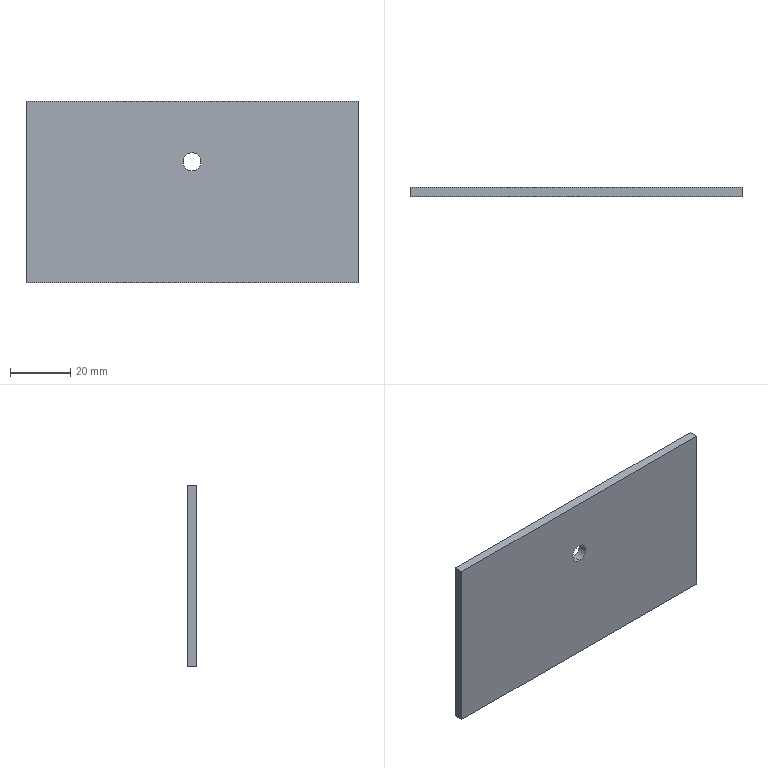Part | SolidWorks | features Extrusion 1 | 1 solid | 8 faces | box 110 x 3 x 60 mm | volume 19715 mm3 | plane 6 | cylinder 2 | commonest cylinder face diameters 6 x2
STEP:
#1=CARTESIAN_POINT('',(0.,3.,7.));
#2=VERTEX_POINT('',#1);
#3=CARTESIAN_POINT('',(0.,3.,13.));
#4=VERTEX_POINT('',#3);
#5=CARTESIAN_POINT('',(0.,3.,10.));
#6=DIRECTION('',(0.,1.,0.));
#7=DIRECTION('',(0.,0.,1.));
#8=AXIS2_PLACEMENT_3D('',#5,#6,#7);
#9=CIRCLE('',#8,3.);
#10=EDGE_CURVE('',#2,#4,#9,.T.);
#11=ORIENTED_EDGE('',*,*,#10,.T.);
#12=CARTESIAN_POINT('',(0.,0.,13.));
#13=VERTEX_POINT('',#12);
#14=CARTESIAN_POINT('',(0.,3.,13.));
#15=DIRECTION('',(0.,-1.,0.));
#16=VECTOR('',#15,1000.);
#17=LINE('',#14,#16);
#18=EDGE_CURVE('',#4,#13,#17,.T.);
#19=ORIENTED_EDGE('',*,*,#18,.T.);
#20=CARTESIAN_POINT('',(0.,0.,7.));
#21=VERTEX_POINT('',#20);
#22=CARTESIAN_POINT('',(0.,0.,10.));
#23=DIRECTION('',(0.,1.,0.));
#24=DIRECTION('',(0.,0.,1.));
#25=AXIS2_PLACEMENT_3D('',#22,#23,#24);
#26=CIRCLE('',#25,3.);
#27=EDGE_CURVE('',#21,#13,#26,.T.);
#28=ORIENTED_EDGE('',*,*,#27,.F.);
#29=CARTESIAN_POINT('',(0.,3.,7.));
#30=DIRECTION('',(0.,-1.,0.));
#31=VECTOR('',#30,1000.);
#32=LINE('',#29,#31);
#33=EDGE_CURVE('',#2,#21,#32,.T.);
#34=ORIENTED_EDGE('',*,*,#33,.F.);
#35=EDGE_LOOP('',(#11,#19,#28,#34));
#36=FACE_OUTER_BOUND('',#35,.T.);
#37=CARTESIAN_POINT('',(0.,3.,10.));
#38=DIRECTION('',(0.,-1.,0.));
#39=DIRECTION('',(0.,0.,-1.));
#40=AXIS2_PLACEMENT_3D('',#37,#38,#39);
#41=CYLINDRICAL_SURFACE('',#40,3.);
#42=ADVANCED_FACE('',(#36),#41,.F.);
#43=CARTESIAN_POINT('',(55.,3.,30.));
#44=VERTEX_POINT('',#43);
#45=CARTESIAN_POINT('',(55.,3.,-30.));
#46=VERTEX_POINT('',#45);
#47=CARTESIAN_POINT('',(55.,3.,30.));
#48=DIRECTION('',(0.,0.,-1.));
#49=VECTOR('',#48,1000.);
#50=LINE('',#47,#49);
#51=EDGE_CURVE('',#44,#46,#50,.T.);
#52=ORIENTED_EDGE('',*,*,#51,.T.);
#53=CARTESIAN_POINT('',(-55.,3.,-30.));
#54=VERTEX_POINT('',#53);
#55=CARTESIAN_POINT('',(-55.,3.,-30.));
#56=DIRECTION('',(-1.,0.,0.));
#57=VECTOR('',#56,1000.);
#58=LINE('',#55,#57);
#59=EDGE_CURVE('',#46,#54,#58,.T.);
#60=ORIENTED_EDGE('',*,*,#59,.T.);
#61=CARTESIAN_POINT('',(-55.,3.,30.));
#62=VERTEX_POINT('',#61);
#63=CARTESIAN_POINT('',(-55.,3.,30.));
#64=DIRECTION('',(0.,0.,1.));
#65=VECTOR('',#64,1000.);
#66=LINE('',#63,#65);
#67=EDGE_CURVE('',#54,#62,#66,.T.);
#68=ORIENTED_EDGE('',*,*,#67,.T.);
#69=CARTESIAN_POINT('',(-55.,3.,30.));
#70=DIRECTION('',(1.,0.,0.));
#71=VECTOR('',#70,1000.);
#72=LINE('',#69,#71);
#73=EDGE_CURVE('',#62,#44,#72,.T.);
#74=ORIENTED_EDGE('',*,*,#73,.T.);
#75=EDGE_LOOP('',(#52,#60,#68,#74));
#76=FACE_OUTER_BOUND('',#75,.T.);
#77=ORIENTED_EDGE('',*,*,#10,.F.);
#78=CARTESIAN_POINT('',(0.,3.,10.));
#79=DIRECTION('',(0.,1.,0.));
#80=DIRECTION('',(0.,0.,1.));
#81=AXIS2_PLACEMENT_3D('',#78,#79,#80);
#82=CIRCLE('',#81,3.);
#83=EDGE_CURVE('',#4,#2,#82,.T.);
#84=ORIENTED_EDGE('',*,*,#83,.F.);
#85=EDGE_LOOP('',(#77,#84));
#86=FACE_BOUND('',#85,.T.);
#87=CARTESIAN_POINT('',(0.,3.,0.));
#88=DIRECTION('',(0.,-1.,0.));
#89=DIRECTION('',(0.,0.,-1.));
#90=AXIS2_PLACEMENT_3D('',#87,#88,#89);
#91=PLANE('',#90);
#92=ADVANCED_FACE('',(#76,#86),#91,.F.);
#93=CARTESIAN_POINT('',(55.,0.,30.));
#94=VERTEX_POINT('',#93);
#95=CARTESIAN_POINT('',(55.,0.,-30.));
#96=VERTEX_POINT('',#95);
#97=CARTESIAN_POINT('',(55.,0.,30.));
#98=DIRECTION('',(0.,0.,-1.));
#99=VECTOR('',#98,1000.);
#100=LINE('',#97,#99);
#101=EDGE_CURVE('',#94,#96,#100,.T.);
#102=ORIENTED_EDGE('',*,*,#101,.F.);
#103=CARTESIAN_POINT('',(-55.,0.,30.));
#104=VERTEX_POINT('',#103);
#105=CARTESIAN_POINT('',(-55.,0.,30.));
#106=DIRECTION('',(1.,0.,0.));
#107=VECTOR('',#106,1000.);
#108=LINE('',#105,#107);
#109=EDGE_CURVE('',#104,#94,#108,.T.);
#110=ORIENTED_EDGE('',*,*,#109,.F.);
#111=CARTESIAN_POINT('',(-55.,0.,-30.));
#112=VERTEX_POINT('',#111);
#113=CARTESIAN_POINT('',(-55.,0.,30.));
#114=DIRECTION('',(0.,0.,1.));
#115=VECTOR('',#114,1000.);
#116=LINE('',#113,#115);
#117=EDGE_CURVE('',#112,#104,#116,.T.);
#118=ORIENTED_EDGE('',*,*,#117,.F.);
#119=CARTESIAN_POINT('',(-55.,0.,-30.));
#120=DIRECTION('',(-1.,0.,0.));
#121=VECTOR('',#120,1000.);
#122=LINE('',#119,#121);
#123=EDGE_CURVE('',#96,#112,#122,.T.);
#124=ORIENTED_EDGE('',*,*,#123,.F.);
#125=EDGE_LOOP('',(#102,#110,#118,#124));
#126=FACE_OUTER_BOUND('',#125,.T.);
#127=ORIENTED_EDGE('',*,*,#27,.T.);
#128=CARTESIAN_POINT('',(0.,0.,10.));
#129=DIRECTION('',(0.,1.,0.));
#130=DIRECTION('',(0.,0.,1.));
#131=AXIS2_PLACEMENT_3D('',#128,#129,#130);
#132=CIRCLE('',#131,3.);
#133=EDGE_CURVE('',#13,#21,#132,.T.);
#134=ORIENTED_EDGE('',*,*,#133,.T.);
#135=EDGE_LOOP('',(#127,#134));
#136=FACE_BOUND('',#135,.T.);
#137=CARTESIAN_POINT('',(0.,0.,0.));
#138=DIRECTION('',(0.,-1.,0.));
#139=DIRECTION('',(0.,0.,-1.));
#140=AXIS2_PLACEMENT_3D('',#137,#138,#139);
#141=PLANE('',#140);
#142=ADVANCED_FACE('',(#126,#136),#141,.T.);
#143=ORIENTED_EDGE('',*,*,#101,.T.);
#144=CARTESIAN_POINT('',(55.,3.,-30.));
#145=DIRECTION('',(0.,-1.,0.));
#146=VECTOR('',#145,1000.);
#147=LINE('',#144,#146);
#148=EDGE_CURVE('',#46,#96,#147,.T.);
#149=ORIENTED_EDGE('',*,*,#148,.F.);
#150=ORIENTED_EDGE('',*,*,#51,.F.);
#151=CARTESIAN_POINT('',(55.,3.,30.));
#152=DIRECTION('',(0.,-1.,0.));
#153=VECTOR('',#152,1000.);
#154=LINE('',#151,#153);
#155=EDGE_CURVE('',#44,#94,#154,.T.);
#156=ORIENTED_EDGE('',*,*,#155,.T.);
#157=EDGE_LOOP('',(#143,#149,#150,#156));
#158=FACE_OUTER_BOUND('',#157,.T.);
#159=CARTESIAN_POINT('',(55.,3.,30.));
#160=DIRECTION('',(-1.,0.,0.));
#161=DIRECTION('',(0.,0.,1.));
#162=AXIS2_PLACEMENT_3D('',#159,#160,#161);
#163=PLANE('',#162);
#164=ADVANCED_FACE('',(#158),#163,.F.);
#165=ORIENTED_EDGE('',*,*,#123,.T.);
#166=CARTESIAN_POINT('',(-55.,3.,-30.));
#167=DIRECTION('',(0.,-1.,0.));
#168=VECTOR('',#167,1000.);
#169=LINE('',#166,#168);
#170=EDGE_CURVE('',#54,#112,#169,.T.);
#171=ORIENTED_EDGE('',*,*,#170,.F.);
#172=ORIENTED_EDGE('',*,*,#59,.F.);
#173=ORIENTED_EDGE('',*,*,#148,.T.);
#174=EDGE_LOOP('',(#165,#171,#172,#173));
#175=FACE_OUTER_BOUND('',#174,.T.);
#176=CARTESIAN_POINT('',(-55.,3.,-30.));
#177=DIRECTION('',(0.,0.,1.));
#178=DIRECTION('',(1.,0.,0.));
#179=AXIS2_PLACEMENT_3D('',#176,#177,#178);
#180=PLANE('',#179);
#181=ADVANCED_FACE('',(#175),#180,.F.);
#182=ORIENTED_EDGE('',*,*,#117,.T.);
#183=CARTESIAN_POINT('',(-55.,3.,30.));
#184=DIRECTION('',(0.,-1.,0.));
#185=VECTOR('',#184,1000.);
#186=LINE('',#183,#185);
#187=EDGE_CURVE('',#62,#104,#186,.T.);
#188=ORIENTED_EDGE('',*,*,#187,.F.);
#189=ORIENTED_EDGE('',*,*,#67,.F.);
#190=ORIENTED_EDGE('',*,*,#170,.T.);
#191=EDGE_LOOP('',(#182,#188,#189,#190));
#192=FACE_OUTER_BOUND('',#191,.T.);
#193=CARTESIAN_POINT('',(-55.,3.,30.));
#194=DIRECTION('',(1.,0.,0.));
#195=DIRECTION('',(0.,0.,-1.));
#196=AXIS2_PLACEMENT_3D('',#193,#194,#195);
#197=PLANE('',#196);
#198=ADVANCED_FACE('',(#192),#197,.F.);
#199=ORIENTED_EDGE('',*,*,#109,.T.);
#200=ORIENTED_EDGE('',*,*,#155,.F.);
#201=ORIENTED_EDGE('',*,*,#73,.F.);
#202=ORIENTED_EDGE('',*,*,#187,.T.);
#203=EDGE_LOOP('',(#199,#200,#201,#202));
#204=FACE_OUTER_BOUND('',#203,.T.);
#205=CARTESIAN_POINT('',(-55.,3.,30.));
#206=DIRECTION('',(0.,0.,-1.));
#207=DIRECTION('',(-1.,0.,0.));
#208=AXIS2_PLACEMENT_3D('',#205,#206,#207);
#209=PLANE('',#208);
#210=ADVANCED_FACE('',(#204),#209,.F.);
#211=ORIENTED_EDGE('',*,*,#18,.F.);
#212=ORIENTED_EDGE('',*,*,#83,.T.);
#213=ORIENTED_EDGE('',*,*,#33,.T.);
#214=ORIENTED_EDGE('',*,*,#133,.F.);
#215=EDGE_LOOP('',(#211,#212,#213,#214));
#216=FACE_OUTER_BOUND('',#215,.T.);
#217=CARTESIAN_POINT('',(0.,3.,10.));
#218=DIRECTION('',(0.,-1.,0.));
#219=DIRECTION('',(0.,0.,-1.));
#220=AXIS2_PLACEMENT_3D('',#217,#218,#219);
#221=CYLINDRICAL_SURFACE('',#220,3.);
#222=ADVANCED_FACE('',(#216),#221,.F.);
#223=CLOSED_SHELL('',(#42,#92,#142,#164,#181,#198,#210,#222));
#224=MANIFOLD_SOLID_BREP('',#223);
#225=CARTESIAN_POINT('',(0.,0.,0.));
#226=DIRECTION('',(0.,0.,1.));
#227=DIRECTION('',(1.,0.,0.));
#228=AXIS2_PLACEMENT_3D('',#225,#226,#227);
#229=(LENGTH_UNIT()NAMED_UNIT(*)SI_UNIT(.MILLI.,.METRE.));
#230=UNCERTAINTY_MEASURE_WITH_UNIT(LENGTH_MEASURE(0.00001),#229,'','');
#231=(NAMED_UNIT(*)PLANE_ANGLE_UNIT()SI_UNIT($,.RADIAN.));
#232=(NAMED_UNIT(*)SI_UNIT($,.STERADIAN.)SOLID_ANGLE_UNIT());
#233=(GEOMETRIC_REPRESENTATION_CONTEXT(3)GLOBAL_UNCERTAINTY_ASSIGNED_CONTEXT((#230))GLOBAL_UNIT_ASSIGNED_CONTEXT((#229,#231,#232))REPRESENTATION_CONTEXT('',''));
#234=ADVANCED_BREP_SHAPE_REPRESENTATION('',(#224,#228),#233);